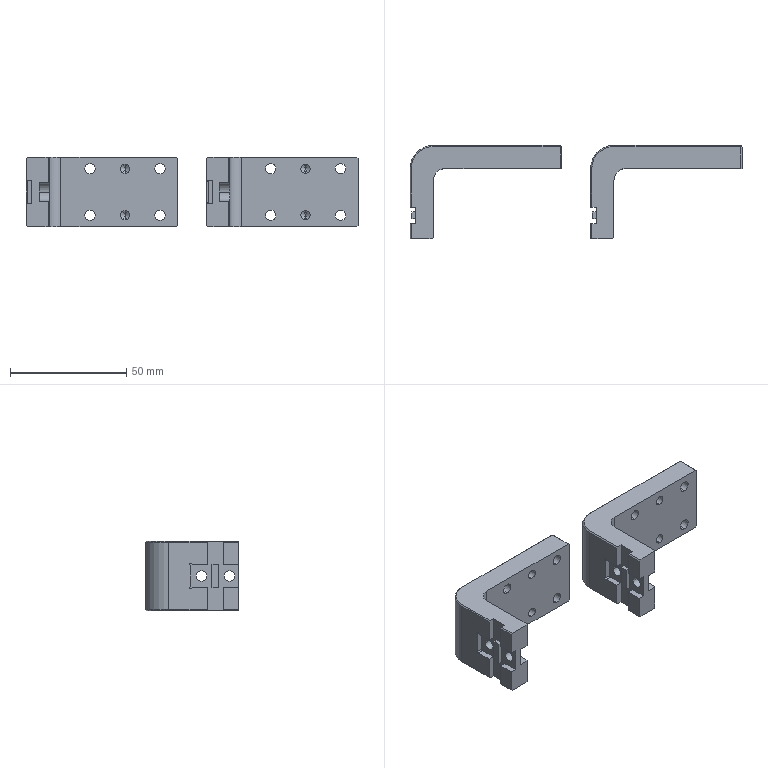NC program | NX | posted with a generic post | part box 142.5 x 40 x 30 mm
Whole program:
N10 G17 G21 G94 G90
(FLOOR_WALL_COPY , TOOL : D80)
N12 T19 M6
N14 G54
N16 G17 G0 G90 X-114.25 Y0. B0. C0. S6500 M3
N18 G43 Z30. H19
N20 Z7.
N22 G94 G1 Z4. F1500.
N24 X-111.25
N26 X111.25
N28 X114.25
N30 Z7.
N32 G0 Z30.
N34 X-114.25
N36 Z6.
N38 G1 Z3.
N40 X-111.25
N42 X111.25
N44 X114.25
N46 Z6.
N48 G0 Z30.
N50 X-114.25
N52 Z5.
N54 G1 Z2.
N56 X-111.25
N58 X111.25
N60 X114.25
N62 Z5.
N64 G0 Z30.
N66 X-114.25
N68 Z4.
N70 G1 Z1.
N72 X-111.25
N74 X111.25
N76 X114.25
N78 Z4.
N80 G0 Z30.
N82 X-114.25
N84 Z3.
N86 G1 Z0.
N88 X-111.25
N90 X111.25
N92 X114.25
N94 Z3.
N96 G0 Z30.
N98 M5
(PLANAR_MILL_COPY_COPY_COPY_COPY_1 , TOOL : D6A45)
N100 T01 M6
N102 G54
N104 G17 G0 G90 X-44.116 Y21.4 B0. C0. S9500 M3
N106 G43 Z30. H1
N108 Z0.5
N110 G94 G1 Z-1. F1250.
N112 G3 X-43.25 Y20.9 R1.
N114 G1 X-16.25
N116 G2 X-5.35 Y10. R10.9
N118 G1 Y-6.55
N120 G2 X-6.25 Y-7.45 R0.9
N122 G1 X-7.85
N124 Y-12.65
N126 X-6.25
N128 G2 X-5.35 Y-13.55 R0.9
N130 G1 Y-20.
N132 G2 X-6.25 Y-20.9 R0.9
N134 G1 X-15.75
N136 G2 X-16.386 Y-20.636 R0.9
N138 G1 X-16.886 Y-20.136
N140 G2 X-17.15 Y-19.5 R0.9
N142 G1 Y5.
N144 G3 X-21.25 Y9.1 R4.1
N146 G1 X-71.25
N148 G2 X-72.15 Y10. R0.9
N150 G1 Y19.
N152 G2 X-70.25 Y20.9 R1.9
N154 G1 X-43.25
N156 G3 X-42.384 Y21.4 R1.
N158 G1 Z0.5
N160 G0 Z30.
N162 X33.384
N164 Z0.5
N166 G1 Z-1.
N168 G3 X34.25 Y20.9 R1.
N170 G1 X61.25
N172 G2 X72.15 Y10. R10.9
N174 G1 Y-6.55
N176 G2 X71.25 Y-7.45 R0.9
N178 G1 X69.65
N180 Y-12.65
N182 X71.25
N184 G2 X72.15 Y-13.55 R0.9
N186 G1 Y-20.
N188 G2 X71.25 Y-20.9 R0.9
N190 G1 X61.75
N192 G2 X61.114 Y-20.636 R0.9
N194 G1 X60.614 Y-20.136
N196 G2 X60.35 Y-19.5 R0.9
N198 G1 Y5.
N200 G3 X56.25 Y9.1 R4.1
N202 G1 X6.25
N204 G2 X5.35 Y10. R0.9
N206 G1 Y19.
N208 G2 X7.25 Y20.9 R1.9
N210 G1 X34.25
N212 G3 X35.116 Y21.4 R1.
N214 G1 Z0.5
N216 G0 Z30.
N218 M5
N220 M2